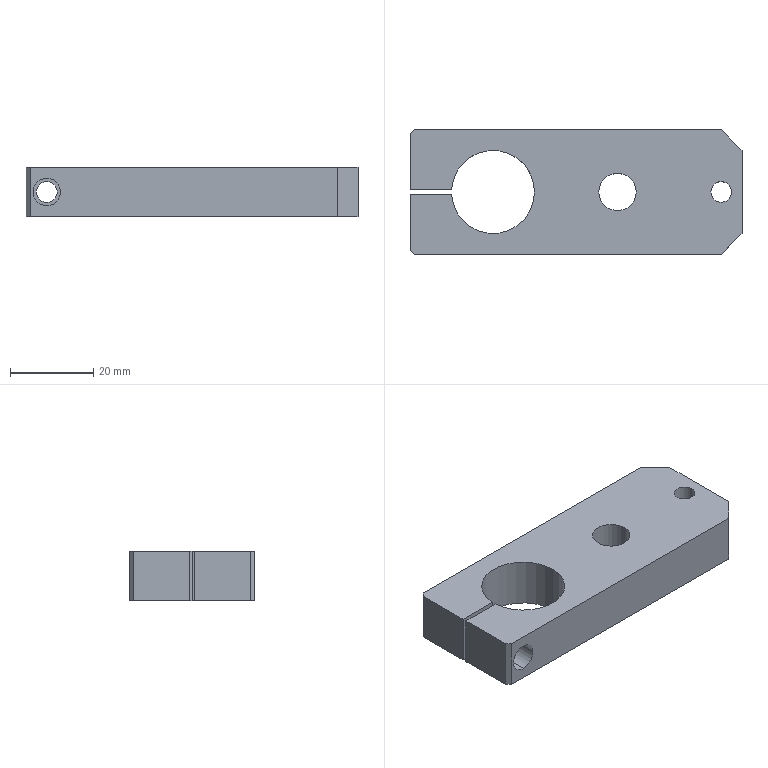Part | STEP file | 001-006-Pre-insertion mechanism buffer mounting plate | 1 solid | 23 faces | box 80 x 30 x 12 mm | volume 22818 mm3 | plane 13 | cylinder 10 | commonest cylinder face diameters 5 x4 6.6 x2 9 x2 20 x2